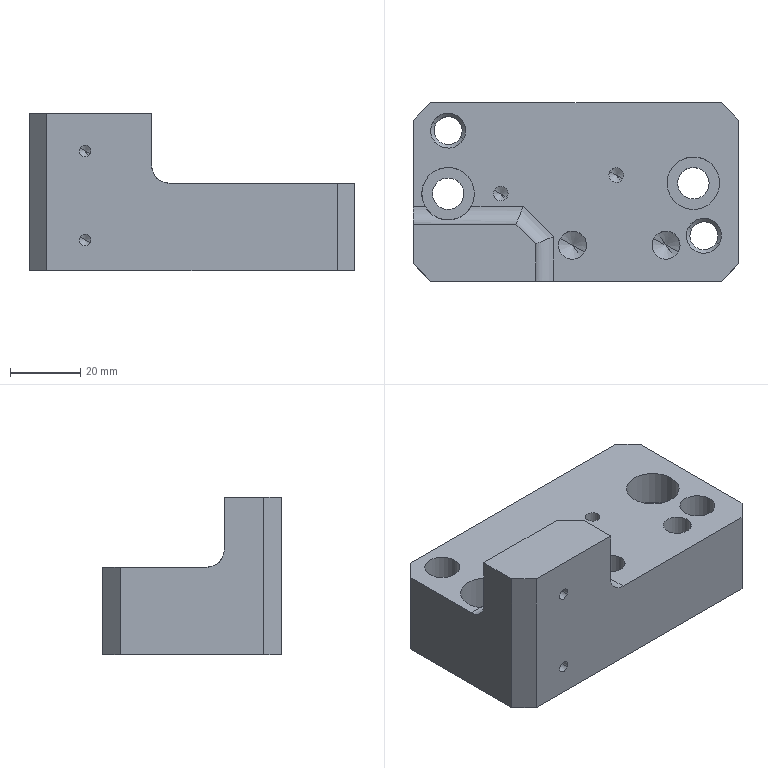Part | CATIA | 1 solid | 63 faces | box 93 x 51 x 45 mm | volume 117179 mm3 | cylinder 31 | plane 16 | cone 16 | commonest cylinder face diameters 8 x8 10 x7 3.3 x4 4.2 x4 9 x4 15 x4